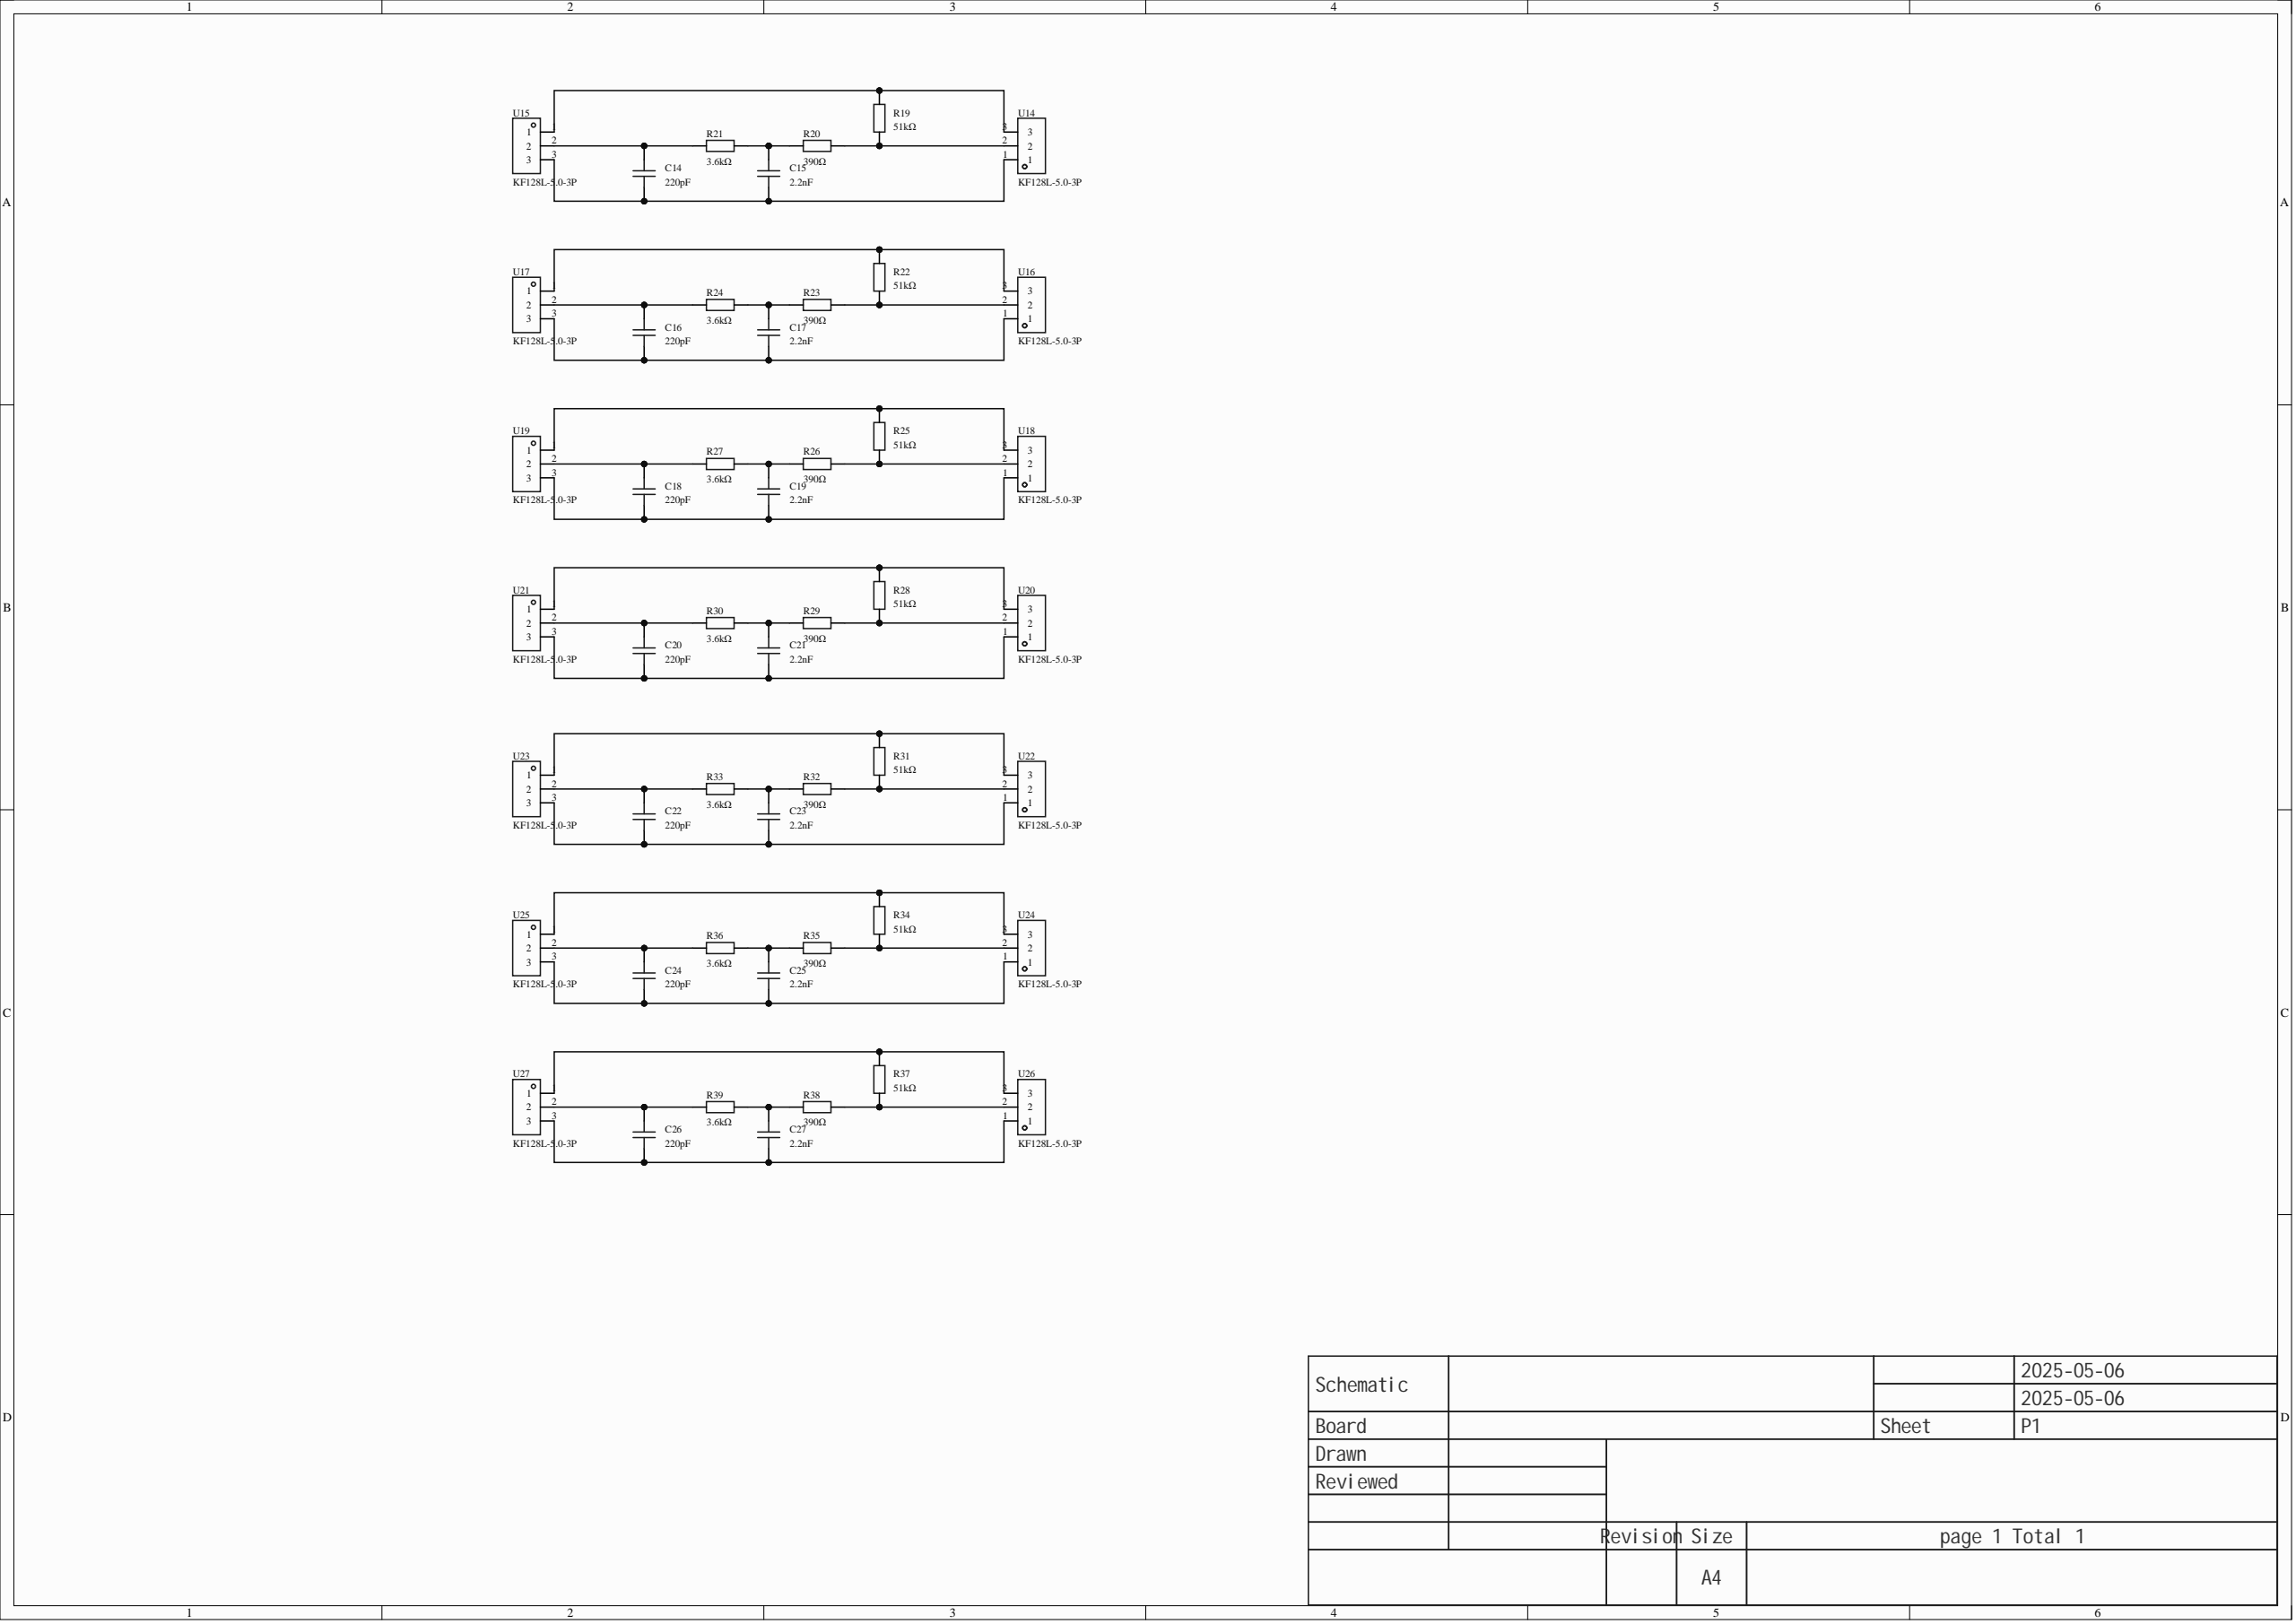Circuit board | Altium Designer | 49 parts | 35 nets
Bill of materials:
Comment,Description,Designator,Footprint,LibRef,Quantity
"220pF","","C14, C16, C18, C20, C22, C24, C26","CAP-TH_L7.2-W4.5-P5.00-D0.5","KP1830122633","7"
"2.2nF","Capacitance:2.2nF;Tolerance:±20%;Voltage(AC):300V;Class:X1,Y2;","C15, C17, C19, C21, C23, C25, C27","CAP-TH_L8.0-W5.0-P7.50-D1.0","DE2E3KY222MA3BU02F","7"
"51kΩ","","R19, R22, R25, R28, R31, R34, R37","Res_1/4W","Res_AXIAL-1/4W","7"
"390Ω","","R20, R23, R26, R29, R32, R35, R38","Res_1/4W","Res_AXIAL-1/4W","7"
"3.6kΩ","","R21, R24, R27, R30, R33, R36, R39","Res_1/4W","Res_AXIAL-1/4W","7"
"KF128L-5.0-3P","Stackable copper RoHS","U14, U15, U16, U17, U18, U19, U20, U21, U22, U23, U24, U25, U26, U27","CONN-TH_3P-P5.00_KF128L-5.0-3P","KF128L-5.0-3P","14"
Netlist (Protel format):
[
C14
CAP-TH_L7.2-W4.5-P5.00-D0.5
220pF



]
[
C15
CAP-TH_L8.0-W5.0-P7.50-D1.0
2.2nF



]
[
C16
CAP-TH_L7.2-W4.5-P5.00-D0.5
220pF



]
[
C17
CAP-TH_L8.0-W5.0-P7.50-D1.0
2.2nF



]
[
C18
CAP-TH_L7.2-W4.5-P5.00-D0.5
220pF



]
[
C19
CAP-TH_L8.0-W5.0-P7.50-D1.0
2.2nF



]
[
C20
CAP-TH_L7.2-W4.5-P5.00-D0.5
220pF



]
[
C21
CAP-TH_L8.0-W5.0-P7.50-D1.0
2.2nF



]
[
C22
CAP-TH_L7.2-W4.5-P5.00-D0.5
220pF



]
[
C23
CAP-TH_L8.0-W5.0-P7.50-D1.0
2.2nF



]
[
C24
CAP-TH_L7.2-W4.5-P5.00-D0.5
220pF



]
[
C25
CAP-TH_L8.0-W5.0-P7.50-D1.0
2.2nF



]
[
C26
CAP-TH_L7.2-W4.5-P5.00-D0.5
220pF



]
[
C27
CAP-TH_L8.0-W5.0-P7.50-D1.0
2.2nF



]
[
R19
Res_1/4W
51kΩ



]
[
R20
Res_1/4W
390Ω



]
[
R21
Res_1/4W
3.6kΩ



]
[
R22
Res_1/4W
51kΩ



]
[
R23
Res_1/4W
390Ω



]
[
R24
Res_1/4W
3.6kΩ



]
[
R25
Res_1/4W
51kΩ



]
[
R26
Res_1/4W
390Ω



]
[
R27
Res_1/4W
3.6kΩ



]
[
R28
Res_1/4W
51kΩ



]
[
R29
Res_1/4W
390Ω



]
[
R30
Res_1/4W
3.6kΩ



]
[
R31
Res_1/4W
51kΩ



]
[
R32
Res_1/4W
390Ω



]
[
R33
Res_1/4W
3.6kΩ



]
[
R34
Res_1/4W
51kΩ



]
[
R35
Res_1/4W
390Ω



]
[
R36
Res_1/4W
3.6kΩ



]
[
R37
Res_1/4W
51kΩ



]
[
R38
Res_1/4W
390Ω



]
[
R39
Res_1/4W
3.6kΩ



]
[
U14
CONN-TH_3P-P5.00_KF128L-5.0-3P
KF128L-5.0-3P



]
[
U15
CONN-TH_3P-P5.00_KF128L-5.0-3P
KF128L-5.0-3P



]
[
U16
CONN-TH_3P-P5.00_KF128L-5.0-3P
KF128L-5.0-3P



]
[
U17
CONN-TH_3P-P5.00_KF128L-5.0-3P
KF128L-5.0-3P



]
[
U18
CONN-TH_3P-P5.00_KF128L-5.0-3P
KF128L-5.0-3P



]
[
U19
CONN-TH_3P-P5.00_KF128L-5.0-3P
KF128L-5.0-3P



]
[
U20
CONN-TH_3P-P5.00_KF128L-5.0-3P
KF128L-5.0-3P



]
[
U21
CONN-TH_3P-P5.00_KF128L-5.0-3P
KF128L-5.0-3P



]
[
U22
CONN-TH_3P-P5.00_KF128L-5.0-3P
KF128L-5.0-3P



]
[
U23
CONN-TH_3P-P5.00_KF128L-5.0-3P
KF128L-5.0-3P



]
[
U24
CONN-TH_3P-P5.00_KF128L-5.0-3P
KF128L-5.0-3P



]
[
U25
CONN-TH_3P-P5.00_KF128L-5.0-3P
KF128L-5.0-3P



]
[
U26
CONN-TH_3P-P5.00_KF128L-5.0-3P
KF128L-5.0-3P



]
[
U27
CONN-TH_3P-P5.00_KF128L-5.0-3P
KF128L-5.0-3P



]
(
NetR37_2
R37-2
U26-3
U27-1
)
(
NetR37_1
R37-1
R38-1
U26-2
)
(
NetR34_2
R34-2
U24-3
U25-1
)
(
NetR34_1
R34-1
R35-1
U24-2
)
(
NetR31_2
R31-2
U22-3
U23-1
)
(
NetR31_1
R31-1
R32-1
U22-2
)
(
NetR28_2
R28-2
U20-3
U21-1
)
(
NetR28_1
R28-1
R29-1
U20-2
)
(
NetR25_2
R25-2
U18-3
U19-1
)
(
NetR25_1
R25-1
R26-1
U18-2
)
(
NetR22_2
R22-2
U16-3
U17-1
)
(
NetR22_1
R22-1
R23-1
U16-2
)
(
NetR19_2
R19-2
U14-3
U15-1
)
(
NetR19_1
R19-1
R20-1
U14-2
)
(
NetC27_2
C27-2
R38-2
R39-1
)
(
NetC26_2
C26-2
R39-2
U27-2
)
(
NetC26_1
C26-1
C27-1
U26-1
U27-3
)
(
NetC25_2
C25-2
R35-2
R36-1
)
(
NetC24_2
C24-2
R36-2
U25-2
)
(
NetC24_1
C24-1
C25-1
U24-1
U25-3
)
(
NetC23_2
C23-2
R32-2
R33-1
)
(
NetC22_2
C22-2
R33-2
U23-2
)
(
NetC22_1
C22-1
C23-1
U22-1
U23-3
)
(
NetC21_2
C21-2
R29-2
R30-1
)
(
NetC20_2
C20-2
R30-2
U21-2
)
(
NetC20_1
C20-1
C21-1
U20-1
U21-3
)
(
NetC19_2
C19-2
R26-2
R27-1
)
(
NetC18_2
C18-2
R27-2
U19-2
)
(
NetC18_1
C18-1
C19-1
U18-1
U19-3
)
(
NetC17_2
C17-2
R23-2
R24-1
)
(
NetC16_2
C16-2
R24-2
U17-2
)
(
NetC16_1
C16-1
C17-1
U16-1
U17-3
)
(
NetC15_2
C15-2
R20-2
R21-1
)
(
NetC14_2
C14-2
R21-2
U15-2
)
(
NetC14_1
C14-1
C15-1
U14-1
U15-3
)